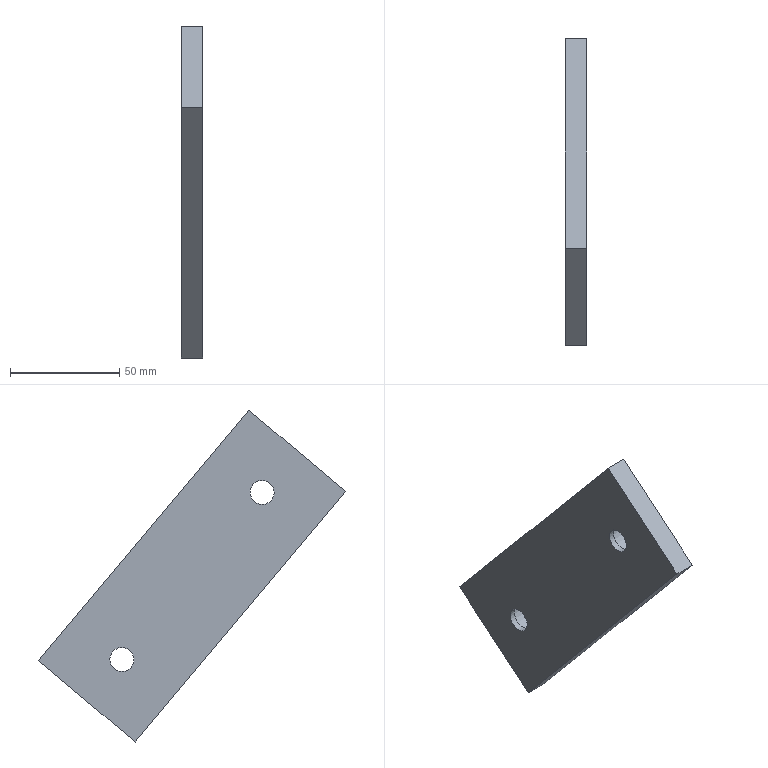Part | NX | features solid 2 | 1 solid | 12 faces | box 10 x 140.849 x 152.188 mm | volume 82975 mm3 | plane 8 | cylinder 4 | commonest cylinder face diameters 11 x2 17.5 x2
STEP:
#1=CARTESIAN_POINT('',(570.,-326.231,-77.93));
#2=VERTEX_POINT('',#1);
#3=CARTESIAN_POINT('',(570.,-370.662,-115.211));
#4=VERTEX_POINT('',#3);
#5=CARTESIAN_POINT('',(570.,-381.004,-123.889));
#6=DIRECTION('',(0.,-0.766,-0.6428));
#7=VECTOR('',#6,1000.);
#8=LINE('',#5,#7);
#9=EDGE_CURVE('',#2,#4,#8,.T.);
#10=ORIENTED_EDGE('',*,*,#9,.F.);
#11=CARTESIAN_POINT('',(560.,-326.231,-77.93));
#12=VERTEX_POINT('',#11);
#13=CARTESIAN_POINT('',(560.,-326.231,-77.93));
#14=DIRECTION('',(1.,0.,0.));
#15=VECTOR('',#14,1000.);
#16=LINE('',#13,#15);
#17=EDGE_CURVE('',#12,#2,#16,.T.);
#18=ORIENTED_EDGE('',*,*,#17,.F.);
#19=CARTESIAN_POINT('',(560.,-370.662,-115.211));
#20=VERTEX_POINT('',#19);
#21=CARTESIAN_POINT('',(560.,-381.004,-123.889));
#22=DIRECTION('',(0.,0.766,0.6428));
#23=VECTOR('',#22,1000.);
#24=LINE('',#21,#23);
#25=EDGE_CURVE('',#12,#20,#24,.F.);
#26=ORIENTED_EDGE('',*,*,#25,.T.);
#27=CARTESIAN_POINT('',(560.,-370.662,-115.211));
#28=DIRECTION('',(1.,0.,0.));
#29=VECTOR('',#28,1000.);
#30=LINE('',#27,#29);
#31=EDGE_CURVE('',#20,#4,#30,.T.);
#32=ORIENTED_EDGE('',*,*,#31,.T.);
#33=EDGE_LOOP('',(#10,#18,#26,#32));
#34=FACE_BOUND('',#33,.T.);
#35=CARTESIAN_POINT('',(560.,-381.004,-123.889));
#36=DIRECTION('',(0.,0.6428,-0.766));
#37=DIRECTION('',(1.,0.,0.));
#38=AXIS2_PLACEMENT_3D('',#35,#36,#37);
#39=PLANE('',#38);
#40=ADVANCED_FACE('',(#34),#39,.F.);
#41=CARTESIAN_POINT('',(570.,-229.813,-192.836));
#42=VERTEX_POINT('',#41);
#43=CARTESIAN_POINT('',(570.,-294.092,-116.232));
#44=DIRECTION('',(0.,-0.6428,0.766));
#45=VECTOR('',#44,1000.);
#46=LINE('',#43,#45);
#47=EDGE_CURVE('',#42,#2,#46,.T.);
#48=ORIENTED_EDGE('',*,*,#47,.F.);
#49=CARTESIAN_POINT('',(560.,-229.813,-192.836));
#50=VERTEX_POINT('',#49);
#51=CARTESIAN_POINT('',(560.,-229.813,-192.836));
#52=DIRECTION('',(1.,0.,0.));
#53=VECTOR('',#52,1000.);
#54=LINE('',#51,#53);
#55=EDGE_CURVE('',#50,#42,#54,.T.);
#56=ORIENTED_EDGE('',*,*,#55,.F.);
#57=CARTESIAN_POINT('',(560.,-294.092,-116.232));
#58=DIRECTION('',(0.,-0.6428,0.766));
#59=VECTOR('',#58,1000.);
#60=LINE('',#57,#59);
#61=EDGE_CURVE('',#50,#12,#60,.T.);
#62=ORIENTED_EDGE('',*,*,#61,.T.);
#63=ORIENTED_EDGE('',*,*,#17,.T.);
#64=EDGE_LOOP('',(#48,#56,#62,#63));
#65=FACE_BOUND('',#64,.T.);
#66=CARTESIAN_POINT('',(560.,-294.092,-116.232));
#67=DIRECTION('',(0.,-0.766,-0.6428));
#68=DIRECTION('',(-1.,0.,0.));
#69=AXIS2_PLACEMENT_3D('',#66,#67,#68);
#70=PLANE('',#69);
#71=ADVANCED_FACE('',(#65),#70,.F.);
#72=CARTESIAN_POINT('',(570.,-274.244,-230.118));
#73=VERTEX_POINT('',#72);
#74=CARTESIAN_POINT('',(570.,-240.155,-201.514));
#75=DIRECTION('',(0.,0.766,0.6428));
#76=VECTOR('',#75,1000.);
#77=LINE('',#74,#76);
#78=EDGE_CURVE('',#73,#42,#77,.T.);
#79=ORIENTED_EDGE('',*,*,#78,.F.);
#80=CARTESIAN_POINT('',(560.,-274.244,-230.118));
#81=VERTEX_POINT('',#80);
#82=CARTESIAN_POINT('',(560.,-274.244,-230.118));
#83=DIRECTION('',(1.,0.,0.));
#84=VECTOR('',#83,1000.);
#85=LINE('',#82,#84);
#86=EDGE_CURVE('',#81,#73,#85,.T.);
#87=ORIENTED_EDGE('',*,*,#86,.F.);
#88=CARTESIAN_POINT('',(560.,-240.155,-201.514));
#89=DIRECTION('',(0.,-0.766,-0.6428));
#90=VECTOR('',#89,1000.);
#91=LINE('',#88,#90);
#92=EDGE_CURVE('',#81,#50,#91,.F.);
#93=ORIENTED_EDGE('',*,*,#92,.T.);
#94=ORIENTED_EDGE('',*,*,#55,.T.);
#95=EDGE_LOOP('',(#79,#87,#93,#94));
#96=FACE_BOUND('',#95,.T.);
#97=CARTESIAN_POINT('',(560.,-240.155,-201.514));
#98=DIRECTION('',(0.,-0.6428,0.766));
#99=DIRECTION('',(-1.,0.,0.));
#100=AXIS2_PLACEMENT_3D('',#97,#98,#99);
#101=PLANE('',#100);
#102=ADVANCED_FACE('',(#96),#101,.F.);
#103=CARTESIAN_POINT('',(570.,-242.105,-268.42));
#104=DIRECTION('',(0.,0.6428,-0.766));
#105=VECTOR('',#104,1000.);
#106=LINE('',#103,#105);
#107=EDGE_CURVE('',#4,#73,#106,.T.);
#108=ORIENTED_EDGE('',*,*,#107,.F.);
#109=ORIENTED_EDGE('',*,*,#31,.F.);
#110=CARTESIAN_POINT('',(560.,-338.523,-153.514));
#111=DIRECTION('',(0.,0.6428,-0.766));
#112=VECTOR('',#111,1000.);
#113=LINE('',#110,#112);
#114=EDGE_CURVE('',#20,#81,#113,.T.);
#115=ORIENTED_EDGE('',*,*,#114,.T.);
#116=ORIENTED_EDGE('',*,*,#86,.T.);
#117=EDGE_LOOP('',(#108,#109,#115,#116));
#118=FACE_BOUND('',#117,.T.);
#119=CARTESIAN_POINT('',(560.,-242.105,-268.42));
#120=DIRECTION('',(0.,0.766,0.6428));
#121=DIRECTION('',(0.,0.6428,-0.766));
#122=AXIS2_PLACEMENT_3D('',#119,#120,#121);
#123=PLANE('',#122);
#124=ADVANCED_FACE('',(#118),#123,.F.);
#125=CARTESIAN_POINT('',(562.7,-326.753,-122.424));
#126=VERTEX_POINT('',#125);
#127=CARTESIAN_POINT('',(562.7,-332.377,-115.722));
#128=DIRECTION('',(-1.,0.,0.));
#129=DIRECTION('',(0.,0.6428,-0.766));
#130=AXIS2_PLACEMENT_3D('',#127,#128,#129);
#131=CIRCLE('',#130,8.75);
#132=EDGE_CURVE('',#126,#126,#131,.T.);
#133=ORIENTED_EDGE('',*,*,#132,.T.);
#134=EDGE_LOOP('',(#133));
#135=FACE_BOUND('',#134,.T.);
#136=CARTESIAN_POINT('',(570.,-339.08,-121.346));
#137=VERTEX_POINT('',#136);
#138=CARTESIAN_POINT('',(570.,-332.377,-115.722));
#139=DIRECTION('',(1.,0.,0.));
#140=DIRECTION('',(0.,-0.766,-0.6428));
#141=AXIS2_PLACEMENT_3D('',#138,#139,#140);
#142=CIRCLE('',#141,8.75);
#143=EDGE_CURVE('',#137,#137,#142,.F.);
#144=ORIENTED_EDGE('',*,*,#143,.F.);
#145=EDGE_LOOP('',(#144));
#146=FACE_BOUND('',#145,.T.);
#147=CARTESIAN_POINT('',(580.,-332.377,-115.722));
#148=DIRECTION('',(-1.,0.,0.));
#149=DIRECTION('',(0.,0.6428,-0.766));
#150=AXIS2_PLACEMENT_3D('',#147,#148,#149);
#151=CYLINDRICAL_SURFACE('',#150,8.75);
#152=ADVANCED_FACE('',(#135,#146),#151,.F.);
#153=CARTESIAN_POINT('',(562.7,-262.474,-199.029));
#154=VERTEX_POINT('',#153);
#155=CARTESIAN_POINT('',(562.7,-268.098,-192.326));
#156=DIRECTION('',(-1.,0.,0.));
#157=DIRECTION('',(0.,0.6428,-0.766));
#158=AXIS2_PLACEMENT_3D('',#155,#156,#157);
#159=CIRCLE('',#158,8.75);
#160=EDGE_CURVE('',#154,#154,#159,.T.);
#161=ORIENTED_EDGE('',*,*,#160,.T.);
#162=EDGE_LOOP('',(#161));
#163=FACE_BOUND('',#162,.T.);
#164=CARTESIAN_POINT('',(570.,-274.801,-197.95));
#165=VERTEX_POINT('',#164);
#166=CARTESIAN_POINT('',(570.,-268.098,-192.326));
#167=DIRECTION('',(1.,0.,0.));
#168=DIRECTION('',(0.,-0.766,-0.6428));
#169=AXIS2_PLACEMENT_3D('',#166,#167,#168);
#170=CIRCLE('',#169,8.75);
#171=EDGE_CURVE('',#165,#165,#170,.F.);
#172=ORIENTED_EDGE('',*,*,#171,.F.);
#173=EDGE_LOOP('',(#172));
#174=FACE_BOUND('',#173,.T.);
#175=CARTESIAN_POINT('',(580.,-268.098,-192.326));
#176=DIRECTION('',(-1.,0.,0.));
#177=DIRECTION('',(0.,0.6428,-0.766));
#178=AXIS2_PLACEMENT_3D('',#175,#176,#177);
#179=CYLINDRICAL_SURFACE('',#178,8.75);
#180=ADVANCED_FACE('',(#163,#174),#179,.F.);
#181=CARTESIAN_POINT('',(560.,-264.563,-196.539));
#182=VERTEX_POINT('',#181);
#183=CARTESIAN_POINT('',(560.,-268.098,-192.326));
#184=DIRECTION('',(-1.,0.,0.));
#185=DIRECTION('',(0.,0.6428,-0.766));
#186=AXIS2_PLACEMENT_3D('',#183,#184,#185);
#187=CIRCLE('',#186,5.5);
#188=EDGE_CURVE('',#182,#182,#187,.T.);
#189=ORIENTED_EDGE('',*,*,#188,.F.);
#190=EDGE_LOOP('',(#189));
#191=FACE_BOUND('',#190,.T.);
#192=CARTESIAN_POINT('',(560.,-328.842,-119.935));
#193=VERTEX_POINT('',#192);
#194=CARTESIAN_POINT('',(560.,-332.377,-115.722));
#195=DIRECTION('',(-1.,0.,0.));
#196=DIRECTION('',(0.,0.6428,-0.766));
#197=AXIS2_PLACEMENT_3D('',#194,#195,#196);
#198=CIRCLE('',#197,5.5);
#199=EDGE_CURVE('',#193,#193,#198,.T.);
#200=ORIENTED_EDGE('',*,*,#199,.F.);
#201=EDGE_LOOP('',(#200));
#202=FACE_BOUND('',#201,.T.);
#203=ORIENTED_EDGE('',*,*,#92,.F.);
#204=ORIENTED_EDGE('',*,*,#114,.F.);
#205=ORIENTED_EDGE('',*,*,#25,.F.);
#206=ORIENTED_EDGE('',*,*,#61,.F.);
#207=EDGE_LOOP('',(#203,#204,#205,#206));
#208=FACE_BOUND('',#207,.T.);
#209=CARTESIAN_POINT('',(560.,-304.434,-124.909));
#210=DIRECTION('',(-1.,0.,0.));
#211=DIRECTION('',(0.,0.6428,-0.766));
#212=AXIS2_PLACEMENT_3D('',#209,#210,#211);
#213=PLANE('',#212);
#214=ADVANCED_FACE('',(#191,#202,#208),#213,.T.);
#215=ORIENTED_EDGE('',*,*,#199,.T.);
#216=EDGE_LOOP('',(#215));
#217=FACE_BOUND('',#216,.T.);
#218=CARTESIAN_POINT('',(562.7,-328.842,-119.935));
#219=VERTEX_POINT('',#218);
#220=CARTESIAN_POINT('',(562.7,-332.377,-115.722));
#221=DIRECTION('',(-1.,0.,0.));
#222=DIRECTION('',(0.,0.6428,-0.766));
#223=AXIS2_PLACEMENT_3D('',#220,#221,#222);
#224=CIRCLE('',#223,5.5);
#225=EDGE_CURVE('',#219,#219,#224,.T.);
#226=ORIENTED_EDGE('',*,*,#225,.F.);
#227=EDGE_LOOP('',(#226));
#228=FACE_BOUND('',#227,.T.);
#229=CARTESIAN_POINT('',(530.,-332.377,-115.722));
#230=DIRECTION('',(-1.,0.,0.));
#231=DIRECTION('',(0.,0.6428,-0.766));
#232=AXIS2_PLACEMENT_3D('',#229,#230,#231);
#233=CYLINDRICAL_SURFACE('',#232,5.5);
#234=ADVANCED_FACE('',(#217,#228),#233,.F.);
#235=ORIENTED_EDGE('',*,*,#225,.T.);
#236=EDGE_LOOP('',(#235));
#237=FACE_BOUND('',#236,.T.);
#238=ORIENTED_EDGE('',*,*,#132,.F.);
#239=EDGE_LOOP('',(#238));
#240=FACE_BOUND('',#239,.T.);
#241=CARTESIAN_POINT('',(562.7,-332.377,-115.722));
#242=DIRECTION('',(-1.,0.,0.));
#243=DIRECTION('',(0.,0.6428,-0.766));
#244=AXIS2_PLACEMENT_3D('',#241,#242,#243);
#245=PLANE('',#244);
#246=ADVANCED_FACE('',(#237,#240),#245,.F.);
#247=ORIENTED_EDGE('',*,*,#188,.T.);
#248=EDGE_LOOP('',(#247));
#249=FACE_BOUND('',#248,.T.);
#250=CARTESIAN_POINT('',(562.7,-264.563,-196.539));
#251=VERTEX_POINT('',#250);
#252=CARTESIAN_POINT('',(562.7,-268.098,-192.326));
#253=DIRECTION('',(-1.,0.,0.));
#254=DIRECTION('',(0.,0.6428,-0.766));
#255=AXIS2_PLACEMENT_3D('',#252,#253,#254);
#256=CIRCLE('',#255,5.5);
#257=EDGE_CURVE('',#251,#251,#256,.T.);
#258=ORIENTED_EDGE('',*,*,#257,.F.);
#259=EDGE_LOOP('',(#258));
#260=FACE_BOUND('',#259,.T.);
#261=CARTESIAN_POINT('',(530.,-268.098,-192.326));
#262=DIRECTION('',(-1.,0.,0.));
#263=DIRECTION('',(0.,0.6428,-0.766));
#264=AXIS2_PLACEMENT_3D('',#261,#262,#263);
#265=CYLINDRICAL_SURFACE('',#264,5.5);
#266=ADVANCED_FACE('',(#249,#260),#265,.F.);
#267=ORIENTED_EDGE('',*,*,#257,.T.);
#268=EDGE_LOOP('',(#267));
#269=FACE_BOUND('',#268,.T.);
#270=ORIENTED_EDGE('',*,*,#160,.F.);
#271=EDGE_LOOP('',(#270));
#272=FACE_BOUND('',#271,.T.);
#273=CARTESIAN_POINT('',(562.7,-268.098,-192.326));
#274=DIRECTION('',(-1.,0.,0.));
#275=DIRECTION('',(0.,0.6428,-0.766));
#276=AXIS2_PLACEMENT_3D('',#273,#274,#275);
#277=PLANE('',#276);
#278=ADVANCED_FACE('',(#269,#272),#277,.F.);
#279=ORIENTED_EDGE('',*,*,#143,.T.);
#280=EDGE_LOOP('',(#279));
#281=FACE_BOUND('',#280,.T.);
#282=ORIENTED_EDGE('',*,*,#171,.T.);
#283=EDGE_LOOP('',(#282));
#284=FACE_BOUND('',#283,.T.);
#285=ORIENTED_EDGE('',*,*,#47,.T.);
#286=ORIENTED_EDGE('',*,*,#9,.T.);
#287=ORIENTED_EDGE('',*,*,#107,.T.);
#288=ORIENTED_EDGE('',*,*,#78,.T.);
#289=EDGE_LOOP('',(#285,#286,#287,#288));
#290=FACE_BOUND('',#289,.T.);
#291=CARTESIAN_POINT('',(570.,-278.44,-201.004));
#292=DIRECTION('',(1.,0.,0.));
#293=DIRECTION('',(0.,-0.766,-0.6428));
#294=AXIS2_PLACEMENT_3D('',#291,#292,#293);
#295=PLANE('',#294);
#296=ADVANCED_FACE('',(#281,#284,#290),#295,.T.);
#297=CLOSED_SHELL('',(#40,#71,#102,#124,#152,#180,#214,#234,#246,#266,#278,#296));
#298=MANIFOLD_SOLID_BREP('',#297);
#299=(LENGTH_UNIT()NAMED_UNIT(*)SI_UNIT(.MILLI.,.METRE.));
#300=UNCERTAINTY_MEASURE_WITH_UNIT(LENGTH_MEASURE(0.00001),#299,'','');
#301=(NAMED_UNIT(*)PLANE_ANGLE_UNIT()SI_UNIT($,.RADIAN.));
#302=(NAMED_UNIT(*)SI_UNIT($,.STERADIAN.)SOLID_ANGLE_UNIT());
#303=(GEOMETRIC_REPRESENTATION_CONTEXT(3)GLOBAL_UNCERTAINTY_ASSIGNED_CONTEXT((#300))GLOBAL_UNIT_ASSIGNED_CONTEXT((#299,#301,#302))REPRESENTATION_CONTEXT('',''));
#304=ADVANCED_BREP_SHAPE_REPRESENTATION('',(#298),#303);